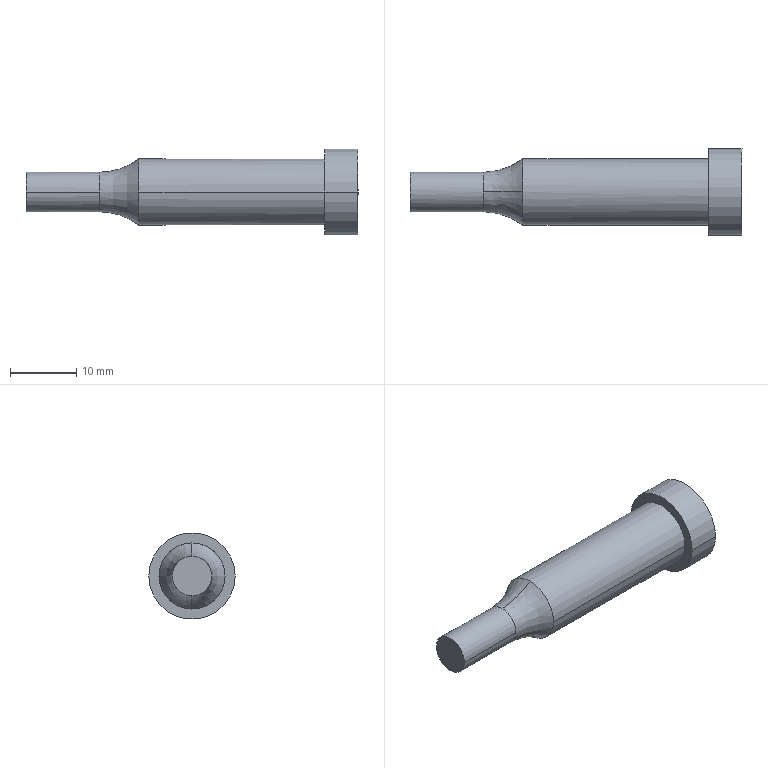Part | STEP file | CHAY 6X10X50.dwg | 1 solid | 11 faces | box 50 x 13 x 13 mm | volume 3399 mm3 | cylinder 6 | plane 3 | spline 2 | commonest cylinder face diameters 5.95 x2 9.95 x2 13 x2
STEP:
#1=CARTESIAN_POINT('',(0.,0.,0.));
#2=DIRECTION('',(0.,0.,1.));
#3=DIRECTION('',(1.,0.,0.));
#4=AXIS2_PLACEMENT_3D('',#1,#2,#3);
#5=CARTESIAN_POINT('',(-39.,2.975,0.));
#6=VERTEX_POINT('',#5);
#7=CARTESIAN_POINT('',(-39.,0.,-2.975));
#8=VERTEX_POINT('',#7);
#9=CARTESIAN_POINT('',(-39.,0.,0.));
#10=DIRECTION('',(-1.,0.,0.));
#11=DIRECTION('',(0.,0.,-1.));
#12=AXIS2_PLACEMENT_3D('',#9,#10,#11);
#13=CIRCLE('',#12,2.975);
#14=CARTESIAN_POINT('',(-39.,0.,-2.975));
#15=CARTESIAN_POINT('',(-39.,5.95,-2.975));
#16=CARTESIAN_POINT('',(-39.,5.95,2.975));
#17=CARTESIAN_POINT('',(-39.,0.,2.975));
#18=CARTESIAN_POINT('',(-36.817,0.,-2.975));
#19=CARTESIAN_POINT('',(-36.817,5.95,-2.975));
#20=CARTESIAN_POINT('',(-36.817,5.95,2.975));
#21=CARTESIAN_POINT('',(-36.817,0.,2.975));
#22=CARTESIAN_POINT('',(-34.746,0.,-3.665));
#23=CARTESIAN_POINT('',(-34.746,7.331,-3.665));
#24=CARTESIAN_POINT('',(-34.746,7.331,3.665));
#25=CARTESIAN_POINT('',(-34.746,0.,3.665));
#26=CARTESIAN_POINT('',(-33.,0.,-4.975));
#27=CARTESIAN_POINT('',(-33.,9.95,-4.975));
#28=CARTESIAN_POINT('',(-33.,9.95,4.975));
#29=CARTESIAN_POINT('',(-33.,0.,4.975));
#30=(BOUNDED_SURFACE()B_SPLINE_SURFACE(3,3,((#14,#15,#16,#17),(#18,#19,#20,#21),(#22,#23,#24,#25),(#26,#27,#28,#29)),.UNSPECIFIED.,.F.,.F.,.F.)B_SPLINE_SURFACE_WITH_KNOTS((4,4),(4,4),(0.,1.),(0.,1.),.PIECEWISE_BEZIER_KNOTS.)GEOMETRIC_REPRESENTATION_ITEM()RATIONAL_B_SPLINE_SURFACE(((1.,0.3333,0.3333,1.),(0.9658,0.3219,0.3219,0.9658),(0.9658,0.3219,0.3219,0.9658),(1.,0.3333,0.3333,1.)))REPRESENTATION_ITEM('')SURFACE());
#31=CARTESIAN_POINT('',(0.,0.5));
#32=CARTESIAN_POINT('',(0.,0.494));
#33=CARTESIAN_POINT('',(0.,0.4822));
#34=CARTESIAN_POINT('',(0.,0.4643));
#35=CARTESIAN_POINT('',(0.,0.4463));
#36=CARTESIAN_POINT('',(0.,0.4281));
#37=CARTESIAN_POINT('',(0.,0.4098));
#38=CARTESIAN_POINT('',(0.,0.3913));
#39=CARTESIAN_POINT('',(0.,0.3724));
#40=CARTESIAN_POINT('',(0.,0.3533));
#41=CARTESIAN_POINT('',(0.,0.3337));
#42=CARTESIAN_POINT('',(0.,0.3136));
#43=CARTESIAN_POINT('',(0.,0.293));
#44=CARTESIAN_POINT('',(0.,0.2718));
#45=CARTESIAN_POINT('',(0.,0.2499));
#46=CARTESIAN_POINT('',(0.,0.2271));
#47=CARTESIAN_POINT('',(0.,0.2035));
#48=CARTESIAN_POINT('',(0.,0.1789));
#49=CARTESIAN_POINT('',(0.,0.1531));
#50=CARTESIAN_POINT('',(0.,0.126));
#51=CARTESIAN_POINT('',(0.,0.09736));
#52=CARTESIAN_POINT('',(0.,0.06707));
#53=CARTESIAN_POINT('',(0.,0.03485));
#54=CARTESIAN_POINT('',(0.,0.0119));
#55=CARTESIAN_POINT('',(0.,0.));
#56=B_SPLINE_CURVE_WITH_KNOTS('',3,(#31,#32,#33,#34,#35,#36,#37,#38,#39,#40,#41,#42,#43,#44,#45,#46,#47,#48,#49,#50,#51,#52,#53,#54,#55),.UNSPECIFIED.,.F.,.F.,(4,1,1,1,1,1,1,1,1,1,1,1,1,1,1,1,1,1,1,1,1,1,4),(4.712,4.784,4.855,4.927,4.998,5.069,5.141,5.212,5.284,5.355,5.426,5.498,5.569,5.641,5.712,5.783,5.855,5.926,5.998,6.069,6.14,6.212,6.283),.QUASI_UNIFORM_KNOTS.);
#57=(GEOMETRIC_REPRESENTATION_CONTEXT(2)PARAMETRIC_REPRESENTATION_CONTEXT()REPRESENTATION_CONTEXT('',''));
#58=DEFINITIONAL_REPRESENTATION('',(#56),#57);
#59=PCURVE('',#30,#58);
#60=CARTESIAN_POINT('',(-44.5,0.,0.));
#61=DIRECTION('',(1.,0.,0.));
#62=DIRECTION('',(0.,1.,0.));
#63=AXIS2_PLACEMENT_3D('',#60,#61,#62);
#64=CYLINDRICAL_SURFACE('',#63,2.975);
#65=CARTESIAN_POINT('',(10.996,5.5));
#66=DIRECTION('',(-1.,0.));
#67=VECTOR('',#66,1.);
#68=LINE('',#65,#67);
#69=(GEOMETRIC_REPRESENTATION_CONTEXT(2)PARAMETRIC_REPRESENTATION_CONTEXT()REPRESENTATION_CONTEXT('',''));
#70=DEFINITIONAL_REPRESENTATION('',(#68),#69);
#71=PCURVE('',#64,#70);
#72=SURFACE_CURVE('',#13,(#59,#71),.PCURVE_S1.);
#73=EDGE_CURVE('',#6,#8,#72,.T.);
#74=ORIENTED_EDGE('',*,*,#73,.T.);
#75=CARTESIAN_POINT('',(-33.,0.,-4.975));
#76=VERTEX_POINT('',#75);
#77=CARTESIAN_POINT('',(-39.,0.,-12.975));
#78=DIRECTION('',(0.,1.,0.));
#79=DIRECTION('',(0.,0.,-1.));
#80=AXIS2_PLACEMENT_3D('',#77,#78,#79);
#81=CIRCLE('',#80,10.);
#82=CARTESIAN_POINT('',(0.,0.));
#83=CARTESIAN_POINT('',(0.01542,0.));
#84=CARTESIAN_POINT('',(0.04618,0.));
#85=CARTESIAN_POINT('',(0.09212,0.));
#86=CARTESIAN_POINT('',(0.1379,0.));
#87=CARTESIAN_POINT('',(0.1835,0.));
#88=CARTESIAN_POINT('',(0.229,0.));
#89=CARTESIAN_POINT('',(0.2743,0.));
#90=CARTESIAN_POINT('',(0.3196,0.));
#91=CARTESIAN_POINT('',(0.3647,0.));
#92=CARTESIAN_POINT('',(0.4099,0.));
#93=CARTESIAN_POINT('',(0.4549,0.));
#94=CARTESIAN_POINT('',(0.5,0.));
#95=CARTESIAN_POINT('',(0.5451,0.));
#96=CARTESIAN_POINT('',(0.5901,0.));
#97=CARTESIAN_POINT('',(0.6353,0.));
#98=CARTESIAN_POINT('',(0.6804,0.));
#99=CARTESIAN_POINT('',(0.7257,0.));
#100=CARTESIAN_POINT('',(0.771,0.));
#101=CARTESIAN_POINT('',(0.8165,0.));
#102=CARTESIAN_POINT('',(0.8621,0.));
#103=CARTESIAN_POINT('',(0.9079,0.));
#104=CARTESIAN_POINT('',(0.9538,0.));
#105=CARTESIAN_POINT('',(0.9846,0.));
#106=CARTESIAN_POINT('',(1.,0.));
#107=B_SPLINE_CURVE_WITH_KNOTS('',3,(#82,#83,#84,#85,#86,#87,#88,#89,#90,#91,#92,#93,#94,#95,#96,#97,#98,#99,#100,#101,#102,#103,#104,#105,#106),.UNSPECIFIED.,.F.,.F.,(4,1,1,1,1,1,1,1,1,1,1,1,1,1,1,1,1,1,1,1,1,1,4),(3.142,3.171,3.2,3.229,3.259,3.288,3.317,3.346,3.376,3.405,3.434,3.463,3.493,3.522,3.551,3.58,3.61,3.639,3.668,3.697,3.727,3.756,3.785),.QUASI_UNIFORM_KNOTS.);
#108=(GEOMETRIC_REPRESENTATION_CONTEXT(2)PARAMETRIC_REPRESENTATION_CONTEXT()REPRESENTATION_CONTEXT('',''));
#109=DEFINITIONAL_REPRESENTATION('',(#107),#108);
#110=PCURVE('',#30,#109);
#111=CARTESIAN_POINT('',(-39.,0.,2.975));
#112=CARTESIAN_POINT('',(-39.,-5.95,2.975));
#113=CARTESIAN_POINT('',(-39.,-5.95,-2.975));
#114=CARTESIAN_POINT('',(-39.,0.,-2.975));
#115=CARTESIAN_POINT('',(-36.817,0.,2.975));
#116=CARTESIAN_POINT('',(-36.817,-5.95,2.975));
#117=CARTESIAN_POINT('',(-36.817,-5.95,-2.975));
#118=CARTESIAN_POINT('',(-36.817,0.,-2.975));
#119=CARTESIAN_POINT('',(-34.746,0.,3.665));
#120=CARTESIAN_POINT('',(-34.746,-7.331,3.665));
#121=CARTESIAN_POINT('',(-34.746,-7.331,-3.665));
#122=CARTESIAN_POINT('',(-34.746,0.,-3.665));
#123=CARTESIAN_POINT('',(-33.,0.,4.975));
#124=CARTESIAN_POINT('',(-33.,-9.95,4.975));
#125=CARTESIAN_POINT('',(-33.,-9.95,-4.975));
#126=CARTESIAN_POINT('',(-33.,0.,-4.975));
#127=(BOUNDED_SURFACE()B_SPLINE_SURFACE(3,3,((#111,#112,#113,#114),(#115,#116,#117,#118),(#119,#120,#121,#122),(#123,#124,#125,#126)),.UNSPECIFIED.,.F.,.F.,.F.)B_SPLINE_SURFACE_WITH_KNOTS((4,4),(4,4),(0.,1.),(0.,1.),.PIECEWISE_BEZIER_KNOTS.)GEOMETRIC_REPRESENTATION_ITEM()RATIONAL_B_SPLINE_SURFACE(((1.,0.3333,0.3333,1.),(0.9658,0.3219,0.3219,0.9658),(0.9658,0.3219,0.3219,0.9658),(1.,0.3333,0.3333,1.)))REPRESENTATION_ITEM('')SURFACE());
#128=CARTESIAN_POINT('',(0.,1.));
#129=CARTESIAN_POINT('',(0.01542,1.));
#130=CARTESIAN_POINT('',(0.04618,1.));
#131=CARTESIAN_POINT('',(0.09212,1.));
#132=CARTESIAN_POINT('',(0.1379,1.));
#133=CARTESIAN_POINT('',(0.1835,1.));
#134=CARTESIAN_POINT('',(0.229,1.));
#135=CARTESIAN_POINT('',(0.2743,1.));
#136=CARTESIAN_POINT('',(0.3196,1.));
#137=CARTESIAN_POINT('',(0.3647,1.));
#138=CARTESIAN_POINT('',(0.4099,1.));
#139=CARTESIAN_POINT('',(0.4549,1.));
#140=CARTESIAN_POINT('',(0.5,1.));
#141=CARTESIAN_POINT('',(0.5451,1.));
#142=CARTESIAN_POINT('',(0.5901,1.));
#143=CARTESIAN_POINT('',(0.6353,1.));
#144=CARTESIAN_POINT('',(0.6804,1.));
#145=CARTESIAN_POINT('',(0.7257,1.));
#146=CARTESIAN_POINT('',(0.771,1.));
#147=CARTESIAN_POINT('',(0.8165,1.));
#148=CARTESIAN_POINT('',(0.8621,1.));
#149=CARTESIAN_POINT('',(0.9079,1.));
#150=CARTESIAN_POINT('',(0.9538,1.));
#151=CARTESIAN_POINT('',(0.9846,1.));
#152=CARTESIAN_POINT('',(1.,1.));
#153=B_SPLINE_CURVE_WITH_KNOTS('',3,(#128,#129,#130,#131,#132,#133,#134,#135,#136,#137,#138,#139,#140,#141,#142,#143,#144,#145,#146,#147,#148,#149,#150,#151,#152),.UNSPECIFIED.,.F.,.F.,(4,1,1,1,1,1,1,1,1,1,1,1,1,1,1,1,1,1,1,1,1,1,4),(3.142,3.171,3.2,3.229,3.259,3.288,3.317,3.346,3.376,3.405,3.434,3.463,3.493,3.522,3.551,3.58,3.61,3.639,3.668,3.697,3.727,3.756,3.785),.QUASI_UNIFORM_KNOTS.);
#154=(GEOMETRIC_REPRESENTATION_CONTEXT(2)PARAMETRIC_REPRESENTATION_CONTEXT()REPRESENTATION_CONTEXT('',''));
#155=DEFINITIONAL_REPRESENTATION('',(#153),#154);
#156=PCURVE('',#127,#155);
#157=SURFACE_CURVE('',#81,(#110,#156),.PCURVE_S1.);
#158=EDGE_CURVE('',#8,#76,#157,.T.);
#159=ORIENTED_EDGE('',*,*,#158,.T.);
#160=CARTESIAN_POINT('',(-33.,4.975,0.));
#161=VERTEX_POINT('',#160);
#162=CARTESIAN_POINT('',(-33.,0.,0.));
#163=DIRECTION('',(1.,0.,0.));
#164=DIRECTION('',(0.,1.,0.));
#165=AXIS2_PLACEMENT_3D('',#162,#163,#164);
#166=CIRCLE('',#165,4.975);
#167=CARTESIAN_POINT('',(1.,0.));
#168=CARTESIAN_POINT('',(1.,0.0119));
#169=CARTESIAN_POINT('',(1.,0.03485));
#170=CARTESIAN_POINT('',(1.,0.06707));
#171=CARTESIAN_POINT('',(1.,0.09736));
#172=CARTESIAN_POINT('',(1.,0.126));
#173=CARTESIAN_POINT('',(1.,0.1531));
#174=CARTESIAN_POINT('',(1.,0.1789));
#175=CARTESIAN_POINT('',(1.,0.2035));
#176=CARTESIAN_POINT('',(1.,0.2271));
#177=CARTESIAN_POINT('',(1.,0.2499));
#178=CARTESIAN_POINT('',(1.,0.2718));
#179=CARTESIAN_POINT('',(1.,0.293));
#180=CARTESIAN_POINT('',(1.,0.3136));
#181=CARTESIAN_POINT('',(1.,0.3337));
#182=CARTESIAN_POINT('',(1.,0.3533));
#183=CARTESIAN_POINT('',(1.,0.3724));
#184=CARTESIAN_POINT('',(1.,0.3913));
#185=CARTESIAN_POINT('',(1.,0.4098));
#186=CARTESIAN_POINT('',(1.,0.4281));
#187=CARTESIAN_POINT('',(1.,0.4463));
#188=CARTESIAN_POINT('',(1.,0.4643));
#189=CARTESIAN_POINT('',(1.,0.4822));
#190=CARTESIAN_POINT('',(1.,0.494));
#191=CARTESIAN_POINT('',(1.,0.5));
#192=B_SPLINE_CURVE_WITH_KNOTS('',3,(#167,#168,#169,#170,#171,#172,#173,#174,#175,#176,#177,#178,#179,#180,#181,#182,#183,#184,#185,#186,#187,#188,#189,#190,#191),.UNSPECIFIED.,.F.,.F.,(4,1,1,1,1,1,1,1,1,1,1,1,1,1,1,1,1,1,1,1,1,1,4),(4.712,4.784,4.855,4.927,4.998,5.069,5.141,5.212,5.284,5.355,5.426,5.498,5.569,5.641,5.712,5.783,5.855,5.926,5.998,6.069,6.14,6.212,6.283),.QUASI_UNIFORM_KNOTS.);
#193=(GEOMETRIC_REPRESENTATION_CONTEXT(2)PARAMETRIC_REPRESENTATION_CONTEXT()REPRESENTATION_CONTEXT('',''));
#194=DEFINITIONAL_REPRESENTATION('',(#192),#193);
#195=PCURVE('',#30,#194);
#196=CARTESIAN_POINT('',(-19.,0.,0.));
#197=DIRECTION('',(1.,0.,0.));
#198=DIRECTION('',(0.,1.,0.));
#199=AXIS2_PLACEMENT_3D('',#196,#197,#198);
#200=CYLINDRICAL_SURFACE('',#199,4.975);
#201=CARTESIAN_POINT('',(0.,-14.));
#202=DIRECTION('',(1.,0.));
#203=VECTOR('',#202,1.);
#204=LINE('',#201,#203);
#205=(GEOMETRIC_REPRESENTATION_CONTEXT(2)PARAMETRIC_REPRESENTATION_CONTEXT()REPRESENTATION_CONTEXT('',''));
#206=DEFINITIONAL_REPRESENTATION('',(#204),#205);
#207=PCURVE('',#200,#206);
#208=SURFACE_CURVE('',#166,(#195,#207),.PCURVE_S1.);
#209=EDGE_CURVE('',#76,#161,#208,.T.);
#210=ORIENTED_EDGE('',*,*,#209,.T.);
#211=CARTESIAN_POINT('',(-33.,0.,4.975));
#212=VERTEX_POINT('',#211);
#213=CARTESIAN_POINT('',(-33.,0.,0.));
#214=DIRECTION('',(1.,0.,0.));
#215=DIRECTION('',(0.,1.,0.));
#216=AXIS2_PLACEMENT_3D('',#213,#214,#215);
#217=CIRCLE('',#216,4.975);
#218=CARTESIAN_POINT('',(1.,0.5));
#219=CARTESIAN_POINT('',(1.,0.506));
#220=CARTESIAN_POINT('',(1.,0.5178));
#221=CARTESIAN_POINT('',(1.,0.5357));
#222=CARTESIAN_POINT('',(1.,0.5537));
#223=CARTESIAN_POINT('',(1.,0.5719));
#224=CARTESIAN_POINT('',(1.,0.5902));
#225=CARTESIAN_POINT('',(1.,0.6087));
#226=CARTESIAN_POINT('',(1.,0.6276));
#227=CARTESIAN_POINT('',(1.,0.6467));
#228=CARTESIAN_POINT('',(1.,0.6663));
#229=CARTESIAN_POINT('',(1.,0.6864));
#230=CARTESIAN_POINT('',(1.,0.707));
#231=CARTESIAN_POINT('',(1.,0.7282));
#232=CARTESIAN_POINT('',(1.,0.7501));
#233=CARTESIAN_POINT('',(1.,0.7729));
#234=CARTESIAN_POINT('',(1.,0.7965));
#235=CARTESIAN_POINT('',(1.,0.8211));
#236=CARTESIAN_POINT('',(1.,0.8469));
#237=CARTESIAN_POINT('',(1.,0.874));
#238=CARTESIAN_POINT('',(1.,0.9026));
#239=CARTESIAN_POINT('',(1.,0.9329));
#240=CARTESIAN_POINT('',(1.,0.9651));
#241=CARTESIAN_POINT('',(1.,0.9881));
#242=CARTESIAN_POINT('',(1.,1.));
#243=B_SPLINE_CURVE_WITH_KNOTS('',3,(#218,#219,#220,#221,#222,#223,#224,#225,#226,#227,#228,#229,#230,#231,#232,#233,#234,#235,#236,#237,#238,#239,#240,#241,#242),.UNSPECIFIED.,.F.,.F.,(4,1,1,1,1,1,1,1,1,1,1,1,1,1,1,1,1,1,1,1,1,1,4),(0.,0.0714,0.1428,0.2142,0.2856,0.357,0.4284,0.4998,0.5712,0.6426,0.714,0.7854,0.8568,0.9282,0.9996,1.071,1.142,1.214,1.285,1.357,1.428,1.499,1.571),.QUASI_UNIFORM_KNOTS.);
#244=(GEOMETRIC_REPRESENTATION_CONTEXT(2)PARAMETRIC_REPRESENTATION_CONTEXT()REPRESENTATION_CONTEXT('',''));
#245=DEFINITIONAL_REPRESENTATION('',(#243),#244);
#246=PCURVE('',#30,#245);
#247=CARTESIAN_POINT('',(-19.,0.,0.));
#248=DIRECTION('',(1.,0.,0.));
#249=DIRECTION('',(0.,1.,0.));
#250=AXIS2_PLACEMENT_3D('',#247,#248,#249);
#251=CYLINDRICAL_SURFACE('',#250,4.975);
#252=CARTESIAN_POINT('',(0.,-14.));
#253=DIRECTION('',(1.,0.));
#254=VECTOR('',#253,1.);
#255=LINE('',#252,#254);
#256=(GEOMETRIC_REPRESENTATION_CONTEXT(2)PARAMETRIC_REPRESENTATION_CONTEXT()REPRESENTATION_CONTEXT('',''));
#257=DEFINITIONAL_REPRESENTATION('',(#255),#256);
#258=PCURVE('',#251,#257);
#259=SURFACE_CURVE('',#217,(#246,#258),.PCURVE_S1.);
#260=EDGE_CURVE('',#161,#212,#259,.T.);
#261=ORIENTED_EDGE('',*,*,#260,.T.);
#262=CARTESIAN_POINT('',(-39.,0.,2.975));
#263=VERTEX_POINT('',#262);
#264=CARTESIAN_POINT('',(-39.,0.,12.975));
#265=DIRECTION('',(0.,-1.,0.));
#266=DIRECTION('',(0.,0.,1.));
#267=AXIS2_PLACEMENT_3D('',#264,#265,#266);
#268=CIRCLE('',#267,10.);
#269=CARTESIAN_POINT('',(0.,1.));
#270=CARTESIAN_POINT('',(0.01542,1.));
#271=CARTESIAN_POINT('',(0.04618,1.));
#272=CARTESIAN_POINT('',(0.09212,1.));
#273=CARTESIAN_POINT('',(0.1379,1.));
#274=CARTESIAN_POINT('',(0.1835,1.));
#275=CARTESIAN_POINT('',(0.229,1.));
#276=CARTESIAN_POINT('',(0.2743,1.));
#277=CARTESIAN_POINT('',(0.3196,1.));
#278=CARTESIAN_POINT('',(0.3647,1.));
#279=CARTESIAN_POINT('',(0.4099,1.));
#280=CARTESIAN_POINT('',(0.4549,1.));
#281=CARTESIAN_POINT('',(0.5,1.));
#282=CARTESIAN_POINT('',(0.5451,1.));
#283=CARTESIAN_POINT('',(0.5901,1.));
#284=CARTESIAN_POINT('',(0.6353,1.));
#285=CARTESIAN_POINT('',(0.6804,1.));
#286=CARTESIAN_POINT('',(0.7257,1.));
#287=CARTESIAN_POINT('',(0.771,1.));
#288=CARTESIAN_POINT('',(0.8165,1.));
#289=CARTESIAN_POINT('',(0.8621,1.));
#290=CARTESIAN_POINT('',(0.9079,1.));
#291=CARTESIAN_POINT('',(0.9538,1.));
#292=CARTESIAN_POINT('',(0.9846,1.));
#293=CARTESIAN_POINT('',(1.,1.));
#294=B_SPLINE_CURVE_WITH_KNOTS('',3,(#269,#270,#271,#272,#273,#274,#275,#276,#277,#278,#279,#280,#281,#282,#283,#284,#285,#286,#287,#288,#289,#290,#291,#292,#293),.UNSPECIFIED.,.F.,.F.,(4,1,1,1,1,1,1,1,1,1,1,1,1,1,1,1,1,1,1,1,1,1,4),(3.142,3.171,3.2,3.229,3.259,3.288,3.317,3.346,3.376,3.405,3.434,3.463,3.493,3.522,3.551,3.58,3.61,3.639,3.668,3.697,3.727,3.756,3.785),.QUASI_UNIFORM_KNOTS.);
#295=(GEOMETRIC_REPRESENTATION_CONTEXT(2)PARAMETRIC_REPRESENTATION_CONTEXT()REPRESENTATION_CONTEXT('',''));
#296=DEFINITIONAL_REPRESENTATION('',(#294),#295);
#297=PCURVE('',#30,#296);
#298=CARTESIAN_POINT('',(0.,0.));
#299=CARTESIAN_POINT('',(0.01542,0.));
#300=CARTESIAN_POINT('',(0.04618,0.));
#301=CARTESIAN_POINT('',(0.09212,0.));
#302=CARTESIAN_POINT('',(0.1379,0.));
#303=CARTESIAN_POINT('',(0.1835,0.));
#304=CARTESIAN_POINT('',(0.229,0.));
#305=CARTESIAN_POINT('',(0.2743,0.));
#306=CARTESIAN_POINT('',(0.3196,0.));
#307=CARTESIAN_POINT('',(0.3647,0.));
#308=CARTESIAN_POINT('',(0.4099,0.));
#309=CARTESIAN_POINT('',(0.4549,0.));
#310=CARTESIAN_POINT('',(0.5,0.));
#311=CARTESIAN_POINT('',(0.5451,0.));
#312=CARTESIAN_POINT('',(0.5901,0.));
#313=CARTESIAN_POINT('',(0.6353,0.));
#314=CARTESIAN_POINT('',(0.6804,0.));
#315=CARTESIAN_POINT('',(0.7257,0.));
#316=CARTESIAN_POINT('',(0.771,0.));
#317=CARTESIAN_POINT('',(0.8165,0.));
#318=CARTESIAN_POINT('',(0.8621,0.));
#319=CARTESIAN_POINT('',(0.9079,0.));
#320=CARTESIAN_POINT('',(0.9538,0.));
#321=CARTESIAN_POINT('',(0.9846,0.));
#322=CARTESIAN_POINT('',(1.,0.));
#323=B_SPLINE_CURVE_WITH_KNOTS('',3,(#298,#299,#300,#301,#302,#303,#304,#305,#306,#307,#308,#309,#310,#311,#312,#313,#314,#315,#316,#317,#318,#319,#320,#321,#322),.UNSPECIFIED.,.F.,.F.,(4,1,1,1,1,1,1,1,1,1,1,1,1,1,1,1,1,1,1,1,1,1,4),(3.142,3.171,3.2,3.229,3.259,3.288,3.317,3.346,3.376,3.405,3.434,3.463,3.493,3.522,3.551,3.58,3.61,3.639,3.668,3.697,3.727,3.756,3.785),.QUASI_UNIFORM_KNOTS.);
#324=(GEOMETRIC_REPRESENTATION_CONTEXT(2)PARAMETRIC_REPRESENTATION_CONTEXT()REPRESENTATION_CONTEXT('',''));
#325=DEFINITIONAL_REPRESENTATION('',(#323),#324);
#326=PCURVE('',#127,#325);
#327=SURFACE_CURVE('',#268,(#297,#326),.PCURVE_S1.);
#328=EDGE_CURVE('',#263,#212,#327,.T.);
#329=ORIENTED_EDGE('',*,*,#328,.F.);
#330=CARTESIAN_POINT('',(-39.,0.,0.));
#331=DIRECTION('',(-1.,0.,0.));
#332=DIRECTION('',(0.,0.,-1.));
#333=AXIS2_PLACEMENT_3D('',#330,#331,#332);
#334=CIRCLE('',#333,2.975);
#335=CARTESIAN_POINT('',(0.,1.));
#336=CARTESIAN_POINT('',(0.,0.9881));
#337=CARTESIAN_POINT('',(0.,0.9651));
#338=CARTESIAN_POINT('',(0.,0.9329));
#339=CARTESIAN_POINT('',(0.,0.9026));
#340=CARTESIAN_POINT('',(0.,0.874));
#341=CARTESIAN_POINT('',(0.,0.8469));
#342=CARTESIAN_POINT('',(0.,0.8211));
#343=CARTESIAN_POINT('',(0.,0.7965));
#344=CARTESIAN_POINT('',(0.,0.7729));
#345=CARTESIAN_POINT('',(0.,0.7501));
#346=CARTESIAN_POINT('',(0.,0.7282));
#347=CARTESIAN_POINT('',(0.,0.707));
#348=CARTESIAN_POINT('',(0.,0.6864));
#349=CARTESIAN_POINT('',(0.,0.6663));
#350=CARTESIAN_POINT('',(0.,0.6467));
#351=CARTESIAN_POINT('',(0.,0.6276));
#352=CARTESIAN_POINT('',(0.,0.6087));
#353=CARTESIAN_POINT('',(0.,0.5902));
#354=CARTESIAN_POINT('',(0.,0.5719));
#355=CARTESIAN_POINT('',(0.,0.5537));
#356=CARTESIAN_POINT('',(0.,0.5357));
#357=CARTESIAN_POINT('',(0.,0.5178));
#358=CARTESIAN_POINT('',(0.,0.506));
#359=CARTESIAN_POINT('',(0.,0.5));
#360=B_SPLINE_CURVE_WITH_KNOTS('',3,(#335,#336,#337,#338,#339,#340,#341,#342,#343,#344,#345,#346,#347,#348,#349,#350,#351,#352,#353,#354,#355,#356,#357,#358,#359),.UNSPECIFIED.,.F.,.F.,(4,1,1,1,1,1,1,1,1,1,1,1,1,1,1,1,1,1,1,1,1,1,4),(3.142,3.213,3.284,3.356,3.427,3.499,3.57,3.641,3.713,3.784,3.856,3.927,3.998,4.07,4.141,4.213,4.284,4.355,4.427,4.498,4.57,4.641,4.712),.QUASI_UNIFORM_KNOTS.);
#361=(GEOMETRIC_REPRESENTATION_CONTEXT(2)PARAMETRIC_REPRESENTATION_CONTEXT()REPRESENTATION_CONTEXT('',''));
#362=DEFINITIONAL_REPRESENTATION('',(#360),#361);
#363=PCURVE('',#30,#362);
#364=CARTESIAN_POINT('',(-44.5,0.,0.));
#365=DIRECTION('',(1.,0.,0.));
#366=DIRECTION('',(0.,1.,0.));
#367=AXIS2_PLACEMENT_3D('',#364,#365,#366);
#368=CYLINDRICAL_SURFACE('',#367,2.975);
#369=CARTESIAN_POINT('',(4.712,5.5));
#370=DIRECTION('',(-1.,0.));
#371=VECTOR('',#370,1.);
#372=LINE('',#369,#371);
#373=(GEOMETRIC_REPRESENTATION_CONTEXT(2)PARAMETRIC_REPRESENTATION_CONTEXT()REPRESENTATION_CONTEXT('',''));
#374=DEFINITIONAL_REPRESENTATION('',(#372),#373);
#375=PCURVE('',#368,#374);
#376=SURFACE_CURVE('',#334,(#363,#375),.PCURVE_S1.);
#377=EDGE_CURVE('',#263,#6,#376,.T.);
#378=ORIENTED_EDGE('',*,*,#377,.T.);
#379=EDGE_LOOP('',(#74,#159,#210,#261,#329,#378));
#380=FACE_BOUND('',#379,.F.);
#381=ADVANCED_FACE('',(#380),#30,.F.);
#382=ORIENTED_EDGE('',*,*,#260,.T.);
#383=CARTESIAN_POINT('',(-33.,-4.975,0.));
#384=VERTEX_POINT('',#383);
#385=CARTESIAN_POINT('',(-33.,0.,0.));
#386=DIRECTION('',(1.,0.,0.));
#387=DIRECTION('',(0.,1.,0.));
#388=AXIS2_PLACEMENT_3D('',#385,#386,#387);
#389=CIRCLE('',#388,4.975);
#390=CARTESIAN_POINT('',(0.,-14.));
#391=DIRECTION('',(1.,0.));
#392=VECTOR('',#391,1.);
#393=LINE('',#390,#392);
#394=(GEOMETRIC_REPRESENTATION_CONTEXT(2)PARAMETRIC_REPRESENTATION_CONTEXT()REPRESENTATION_CONTEXT('',''));
#395=DEFINITIONAL_REPRESENTATION('',(#393),#394);
#396=PCURVE('',#251,#395);
#397=CARTESIAN_POINT('',(1.,0.));
#398=CARTESIAN_POINT('',(1.,0.0119));
#399=CARTESIAN_POINT('',(1.,0.03485));
#400=CARTESIAN_POINT('',(1.,0.06707));
#401=CARTESIAN_POINT('',(1.,0.09736));
#402=CARTESIAN_POINT('',(1.,0.126));
#403=CARTESIAN_POINT('',(1.,0.1531));
#404=CARTESIAN_POINT('',(1.,0.1789));
#405=CARTESIAN_POINT('',(1.,0.2035));
#406=CARTESIAN_POINT('',(1.,0.2271));
#407=CARTESIAN_POINT('',(1.,0.2499));
#408=CARTESIAN_POINT('',(1.,0.2718));
#409=CARTESIAN_POINT('',(1.,0.293));
#410=CARTESIAN_POINT('',(1.,0.3136));
#411=CARTESIAN_POINT('',(1.,0.3337));
#412=CARTESIAN_POINT('',(1.,0.3533));
#413=CARTESIAN_POINT('',(1.,0.3724));
#414=CARTESIAN_POINT('',(1.,0.3913));
#415=CARTESIAN_POINT('',(1.,0.4098));
#416=CARTESIAN_POINT('',(1.,0.4281));
#417=CARTESIAN_POINT('',(1.,0.4463));
#418=CARTESIAN_POINT('',(1.,0.4643));
#419=CARTESIAN_POINT('',(1.,0.4822));
#420=CARTESIAN_POINT('',(1.,0.494));
#421=CARTESIAN_POINT('',(1.,0.5));
#422=B_SPLINE_CURVE_WITH_KNOTS('',3,(#397,#398,#399,#400,#401,#402,#403,#404,#405,#406,#407,#408,#409,#410,#411,#412,#413,#414,#415,#416,#417,#418,#419,#420,#421),.UNSPECIFIED.,.F.,.F.,(4,1,1,1,1,1,1,1,1,1,1,1,1,1,1,1,1,1,1,1,1,1,4),(1.571,1.642,1.714,1.785,1.856,1.928,1.999,2.071,2.142,2.213,2.285,2.356,2.428,2.499,2.57,2.642,2.713,2.785,2.856,2.927,2.999,3.07,3.142),.QUASI_UNIFORM_KNOTS.);
#423=(GEOMETRIC_REPRESENTATION_CONTEXT(2)PARAMETRIC_REPRESENTATION_CONTEXT()REPRESENTATION_CONTEXT('',''));
#424=DEFINITIONAL_REPRESENTATION('',(#422),#423);
#425=PCURVE('',#127,#424);
#426=SURFACE_CURVE('',#389,(#396,#425),.PCURVE_S1.);
#427=EDGE_CURVE('',#212,#384,#426,.T.);
#428=ORIENTED_EDGE('',*,*,#427,.T.);
#429=CARTESIAN_POINT('',(-5.,-4.975,0.));
#430=VERTEX_POINT('',#429);
#431=CARTESIAN_POINT('',(-19.,-4.975,0.));
#432=DIRECTION('',(1.,0.,0.));
#433=VECTOR('',#432,1.);
#434=LINE('',#431,#433);
#435=CARTESIAN_POINT('',(3.142,0.));
#436=DIRECTION('',(0.,1.));
#437=VECTOR('',#436,1.);
#438=LINE('',#435,#437);
#439=(GEOMETRIC_REPRESENTATION_CONTEXT(2)PARAMETRIC_REPRESENTATION_CONTEXT()REPRESENTATION_CONTEXT('',''));
#440=DEFINITIONAL_REPRESENTATION('',(#438),#439);
#441=PCURVE('',#251,#440);
#442=CARTESIAN_POINT('',(3.142,0.));
#443=DIRECTION('',(0.,1.));
#444=VECTOR('',#443,1.);
#445=LINE('',#442,#444);
#446=(GEOMETRIC_REPRESENTATION_CONTEXT(2)PARAMETRIC_REPRESENTATION_CONTEXT()REPRESENTATION_CONTEXT('',''));
#447=DEFINITIONAL_REPRESENTATION('',(#445),#446);
#448=PCURVE('',#200,#447);
#449=SURFACE_CURVE('',#434,(#441,#448),.PCURVE_S1.);
#450=EDGE_CURVE('',#384,#430,#449,.T.);
#451=ORIENTED_EDGE('',*,*,#450,.T.);
#452=CARTESIAN_POINT('',(-5.,4.975,0.));
#453=VERTEX_POINT('',#452);
#454=CARTESIAN_POINT('',(-5.,0.,0.));
#455=DIRECTION('',(-1.,0.,0.));
#456=DIRECTION('',(0.,1.,0.));
#457=AXIS2_PLACEMENT_3D('',#454,#455,#456);
#458=CIRCLE('',#457,4.975);
#459=CARTESIAN_POINT('',(6.283,14.));
#460=DIRECTION('',(-1.,0.));
#461=VECTOR('',#460,1.);
#462=LINE('',#459,#461);
#463=(GEOMETRIC_REPRESENTATION_CONTEXT(2)PARAMETRIC_REPRESENTATION_CONTEXT()REPRESENTATION_CONTEXT('',''));
#464=DEFINITIONAL_REPRESENTATION('',(#462),#463);
#465=PCURVE('',#251,#464);
#466=CARTESIAN_POINT('',(-5.,5.737,0.));
#467=DIRECTION('',(-1.,0.,0.));
#468=DIRECTION('',(0.,0.,1.));
#469=AXIS2_PLACEMENT_3D('',#466,#467,#468);
#470=PLANE('',#469);
#471=CARTESIAN_POINT('',(0.,-5.737));
#472=DIRECTION('',(0.,1.));
#473=AXIS2_PLACEMENT_2D('',#471,#472);
#474=CIRCLE('',#473,4.975);
#475=(GEOMETRIC_REPRESENTATION_CONTEXT(2)PARAMETRIC_REPRESENTATION_CONTEXT()REPRESENTATION_CONTEXT('',''));
#476=DEFINITIONAL_REPRESENTATION('',(#474),#475);
#477=PCURVE('',#470,#476);
#478=SURFACE_CURVE('',#458,(#465,#477),.PCURVE_S1.);
#479=EDGE_CURVE('',#430,#453,#478,.T.);
#480=ORIENTED_EDGE('',*,*,#479,.T.);
#481=CARTESIAN_POINT('',(-19.,4.975,0.));
#482=DIRECTION('',(1.,0.,0.));
#483=VECTOR('',#482,1.);
#484=LINE('',#481,#483);
#485=CARTESIAN_POINT('',(0.,0.));
#486=DIRECTION('',(0.,1.));
#487=VECTOR('',#486,1.);
#488=LINE('',#485,#487);
#489=(GEOMETRIC_REPRESENTATION_CONTEXT(2)PARAMETRIC_REPRESENTATION_CONTEXT()REPRESENTATION_CONTEXT('',''));
#490=DEFINITIONAL_REPRESENTATION('',(#488),#489);
#491=PCURVE('',#251,#490);
#492=CARTESIAN_POINT('',(6.283,0.));
#493=DIRECTION('',(0.,1.));
#494=VECTOR('',#493,1.);
#495=LINE('',#492,#494);
#496=(GEOMETRIC_REPRESENTATION_CONTEXT(2)PARAMETRIC_REPRESENTATION_CONTEXT()REPRESENTATION_CONTEXT('',''));
#497=DEFINITIONAL_REPRESENTATION('',(#495),#496);
#498=PCURVE('',#200,#497);
#499=SURFACE_CURVE('',#484,(#491,#498),.PCURVE_S1.);
#500=EDGE_CURVE('',#161,#453,#499,.T.);
#501=ORIENTED_EDGE('',*,*,#500,.F.);
#502=EDGE_LOOP('',(#382,#428,#451,#480,#501));
#503=FACE_BOUND('',#502,.T.);
#504=ADVANCED_FACE('',(#503),#251,.T.);
#505=CARTESIAN_POINT('',(-50.,2.975,0.));
#506=VERTEX_POINT('',#505);
#507=CARTESIAN_POINT('',(-50.,-2.975,0.));
#508=VERTEX_POINT('',#507);
#509=CARTESIAN_POINT('',(-50.,0.,0.));
#510=DIRECTION('',(1.,0.,0.));
#511=DIRECTION('',(0.,1.,0.));
#512=AXIS2_PLACEMENT_3D('',#509,#510,#511);
#513=CIRCLE('',#512,2.975);
#514=CARTESIAN_POINT('',(0.,-5.5));
#515=DIRECTION('',(1.,0.));
#516=VECTOR('',#515,1.);
#517=LINE('',#514,#516);
#518=(GEOMETRIC_REPRESENTATION_CONTEXT(2)PARAMETRIC_REPRESENTATION_CONTEXT()REPRESENTATION_CONTEXT('',''));
#519=DEFINITIONAL_REPRESENTATION('',(#517),#518);
#520=PCURVE('',#368,#519);
#521=CARTESIAN_POINT('',(-50.,1.487,0.));
#522=DIRECTION('',(-1.,0.,0.));
#523=DIRECTION('',(0.,0.,1.));
#524=AXIS2_PLACEMENT_3D('',#521,#522,#523);
#525=PLANE('',#524);
#526=CARTESIAN_POINT('',(0.,1.487));
#527=CARTESIAN_POINT('',(5.153,1.487));
#528=CARTESIAN_POINT('',(2.576,-2.975));
#529=CARTESIAN_POINT('',(0.,-7.437));
#530=CARTESIAN_POINT('',(-2.576,-2.975));
#531=CARTESIAN_POINT('',(-5.153,1.487));
#532=CARTESIAN_POINT('',(0.,1.487));
#533=(BOUNDED_CURVE()B_SPLINE_CURVE(2,(#526,#527,#528,#529,#530,#531,#532),.UNSPECIFIED.,.T.,.F.)B_SPLINE_CURVE_WITH_KNOTS((1,2,2,2,2,1),(-2.094,0.,2.094,4.189,6.283,8.378),.UNSPECIFIED.)CURVE()GEOMETRIC_REPRESENTATION_ITEM()RATIONAL_B_SPLINE_CURVE((1.,0.5,1.,0.5,1.,0.5,1.))REPRESENTATION_ITEM(''));
#534=(GEOMETRIC_REPRESENTATION_CONTEXT(2)PARAMETRIC_REPRESENTATION_CONTEXT()REPRESENTATION_CONTEXT('',''));
#535=DEFINITIONAL_REPRESENTATION('',(#533),#534);
#536=PCURVE('',#525,#535);
#537=SURFACE_CURVE('',#513,(#520,#536),.PCURVE_S1.);
#538=EDGE_CURVE('',#506,#508,#537,.T.);
#539=ORIENTED_EDGE('',*,*,#538,.T.);
#540=CARTESIAN_POINT('',(-39.,-2.975,0.));
#541=VERTEX_POINT('',#540);
#542=CARTESIAN_POINT('',(-44.5,-2.975,0.));
#543=DIRECTION('',(1.,0.,0.));
#544=VECTOR('',#543,1.);
#545=LINE('',#542,#544);
#546=CARTESIAN_POINT('',(3.142,0.));
#547=DIRECTION('',(0.,1.));
#548=VECTOR('',#547,1.);
#549=LINE('',#546,#548);
#550=(GEOMETRIC_REPRESENTATION_CONTEXT(2)PARAMETRIC_REPRESENTATION_CONTEXT()REPRESENTATION_CONTEXT('',''));
#551=DEFINITIONAL_REPRESENTATION('',(#549),#550);
#552=PCURVE('',#368,#551);
#553=CARTESIAN_POINT('',(3.142,0.));
#554=DIRECTION('',(0.,1.));
#555=VECTOR('',#554,1.);
#556=LINE('',#553,#555);
#557=(GEOMETRIC_REPRESENTATION_CONTEXT(2)PARAMETRIC_REPRESENTATION_CONTEXT()REPRESENTATION_CONTEXT('',''));
#558=DEFINITIONAL_REPRESENTATION('',(#556),#557);
#559=PCURVE('',#64,#558);
#560=SURFACE_CURVE('',#545,(#552,#559),.PCURVE_S1.);
#561=EDGE_CURVE('',#508,#541,#560,.T.);
#562=ORIENTED_EDGE('',*,*,#561,.T.);
#563=CARTESIAN_POINT('',(-39.,0.,0.));
#564=DIRECTION('',(-1.,0.,0.));
#565=DIRECTION('',(0.,0.,-1.));
#566=AXIS2_PLACEMENT_3D('',#563,#564,#565);
#567=CIRCLE('',#566,2.975);
#568=CARTESIAN_POINT('',(4.712,5.5));
#569=DIRECTION('',(-1.,0.));
#570=VECTOR('',#569,1.);
#571=LINE('',#568,#570);
#572=(GEOMETRIC_REPRESENTATION_CONTEXT(2)PARAMETRIC_REPRESENTATION_CONTEXT()REPRESENTATION_CONTEXT('',''));
#573=DEFINITIONAL_REPRESENTATION('',(#571),#572);
#574=PCURVE('',#368,#573);
#575=CARTESIAN_POINT('',(0.,0.5));
#576=CARTESIAN_POINT('',(0.,0.494));
#577=CARTESIAN_POINT('',(0.,0.4822));
#578=CARTESIAN_POINT('',(0.,0.4643));
#579=CARTESIAN_POINT('',(0.,0.4463));
#580=CARTESIAN_POINT('',(0.,0.4281));
#581=CARTESIAN_POINT('',(0.,0.4098));
#582=CARTESIAN_POINT('',(0.,0.3913));
#583=CARTESIAN_POINT('',(0.,0.3724));
#584=CARTESIAN_POINT('',(0.,0.3533));
#585=CARTESIAN_POINT('',(0.,0.3337));
#586=CARTESIAN_POINT('',(0.,0.3136));
#587=CARTESIAN_POINT('',(0.,0.293));
#588=CARTESIAN_POINT('',(0.,0.2718));
#589=CARTESIAN_POINT('',(0.,0.2499));
#590=CARTESIAN_POINT('',(0.,0.2271));
#591=CARTESIAN_POINT('',(0.,0.2035));
#592=CARTESIAN_POINT('',(0.,0.1789));
#593=CARTESIAN_POINT('',(0.,0.1531));
#594=CARTESIAN_POINT('',(0.,0.126));
#595=CARTESIAN_POINT('',(0.,0.09736));
#596=CARTESIAN_POINT('',(0.,0.06707));
#597=CARTESIAN_POINT('',(0.,0.03485));
#598=CARTESIAN_POINT('',(0.,0.0119));
#599=CARTESIAN_POINT('',(0.,0.));
#600=B_SPLINE_CURVE_WITH_KNOTS('',3,(#575,#576,#577,#578,#579,#580,#581,#582,#583,#584,#585,#586,#587,#588,#589,#590,#591,#592,#593,#594,#595,#596,#597,#598,#599),.UNSPECIFIED.,.F.,.F.,(4,1,1,1,1,1,1,1,1,1,1,1,1,1,1,1,1,1,1,1,1,1,4),(1.571,1.642,1.714,1.785,1.856,1.928,1.999,2.071,2.142,2.213,2.285,2.356,2.428,2.499,2.57,2.642,2.713,2.785,2.856,2.927,2.999,3.07,3.142),.QUASI_UNIFORM_KNOTS.);
#601=(GEOMETRIC_REPRESENTATION_CONTEXT(2)PARAMETRIC_REPRESENTATION_CONTEXT()REPRESENTATION_CONTEXT('',''));
#602=DEFINITIONAL_REPRESENTATION('',(#600),#601);
#603=PCURVE('',#127,#602);
#604=SURFACE_CURVE('',#567,(#574,#603),.PCURVE_S1.);
#605=EDGE_CURVE('',#541,#263,#604,.T.);
#606=ORIENTED_EDGE('',*,*,#605,.T.);
#607=ORIENTED_EDGE('',*,*,#377,.T.);
#608=CARTESIAN_POINT('',(-44.5,2.975,0.));
#609=DIRECTION('',(1.,0.,0.));
#610=VECTOR('',#609,1.);
#611=LINE('',#608,#610);
#612=CARTESIAN_POINT('',(0.,0.));
#613=DIRECTION('',(0.,1.));
#614=VECTOR('',#613,1.);
#615=LINE('',#612,#614);
#616=(GEOMETRIC_REPRESENTATION_CONTEXT(2)PARAMETRIC_REPRESENTATION_CONTEXT()REPRESENTATION_CONTEXT('',''));
#617=DEFINITIONAL_REPRESENTATION('',(#615),#616);
#618=PCURVE('',#368,#617);
#619=CARTESIAN_POINT('',(6.283,0.));
#620=DIRECTION('',(0.,1.));
#621=VECTOR('',#620,1.);
#622=LINE('',#619,#621);
#623=(GEOMETRIC_REPRESENTATION_CONTEXT(2)PARAMETRIC_REPRESENTATION_CONTEXT()REPRESENTATION_CONTEXT('',''));
#624=DEFINITIONAL_REPRESENTATION('',(#622),#623);
#625=PCURVE('',#64,#624);
#626=SURFACE_CURVE('',#611,(#618,#625),.PCURVE_S1.);
#627=EDGE_CURVE('',#506,#6,#626,.T.);
#628=ORIENTED_EDGE('',*,*,#627,.F.);
#629=EDGE_LOOP('',(#539,#562,#606,#607,#628));
#630=FACE_BOUND('',#629,.T.);
#631=ADVANCED_FACE('',(#630),#368,.T.);
#632=CARTESIAN_POINT('',(-5.,-6.5,0.));
#633=VERTEX_POINT('',#632);
#634=CARTESIAN_POINT('',(-5.,6.5,0.));
#635=VERTEX_POINT('',#634);
#636=CARTESIAN_POINT('',(-5.,0.,0.));
#637=DIRECTION('',(-1.,0.,0.));
#638=DIRECTION('',(0.,1.,0.));
#639=AXIS2_PLACEMENT_3D('',#636,#637,#638);
#640=CIRCLE('',#639,6.5);
#641=CARTESIAN_POINT('',(-2.5,0.,0.));
#642=DIRECTION('',(1.,0.,0.));
#643=DIRECTION('',(0.,1.,0.));
#644=AXIS2_PLACEMENT_3D('',#641,#642,#643);
#645=CYLINDRICAL_SURFACE('',#644,6.5);
#646=CARTESIAN_POINT('',(6.283,-2.5));
#647=DIRECTION('',(-1.,0.));
#648=VECTOR('',#647,1.);
#649=LINE('',#646,#648);
#650=(GEOMETRIC_REPRESENTATION_CONTEXT(2)PARAMETRIC_REPRESENTATION_CONTEXT()REPRESENTATION_CONTEXT('',''));
#651=DEFINITIONAL_REPRESENTATION('',(#649),#650);
#652=PCURVE('',#645,#651);
#653=CARTESIAN_POINT('',(0.,-5.737));
#654=DIRECTION('',(0.,1.));
#655=AXIS2_PLACEMENT_2D('',#653,#654);
#656=CIRCLE('',#655,6.5);
#657=(GEOMETRIC_REPRESENTATION_CONTEXT(2)PARAMETRIC_REPRESENTATION_CONTEXT()REPRESENTATION_CONTEXT('',''));
#658=DEFINITIONAL_REPRESENTATION('',(#656),#657);
#659=PCURVE('',#470,#658);
#660=SURFACE_CURVE('',#640,(#652,#659),.PCURVE_S1.);
#661=EDGE_CURVE('',#633,#635,#660,.T.);
#662=ORIENTED_EDGE('',*,*,#661,.F.);
#663=CARTESIAN_POINT('',(0.,-6.5,0.));
#664=VERTEX_POINT('',#663);
#665=CARTESIAN_POINT('',(-2.5,-6.5,0.));
#666=DIRECTION('',(1.,0.,0.));
#667=VECTOR('',#666,1.);
#668=LINE('',#665,#667);
#669=CARTESIAN_POINT('',(3.142,0.));
#670=DIRECTION('',(0.,1.));
#671=VECTOR('',#670,1.);
#672=LINE('',#669,#671);
#673=(GEOMETRIC_REPRESENTATION_CONTEXT(2)PARAMETRIC_REPRESENTATION_CONTEXT()REPRESENTATION_CONTEXT('',''));
#674=DEFINITIONAL_REPRESENTATION('',(#672),#673);
#675=PCURVE('',#645,#674);
#676=CARTESIAN_POINT('',(-2.5,0.,0.));
#677=DIRECTION('',(1.,0.,0.));
#678=DIRECTION('',(0.,1.,0.));
#679=AXIS2_PLACEMENT_3D('',#676,#677,#678);
#680=CYLINDRICAL_SURFACE('',#679,6.5);
#681=CARTESIAN_POINT('',(3.142,0.));
#682=DIRECTION('',(0.,1.));
#683=VECTOR('',#682,1.);
#684=LINE('',#681,#683);
#685=(GEOMETRIC_REPRESENTATION_CONTEXT(2)PARAMETRIC_REPRESENTATION_CONTEXT()REPRESENTATION_CONTEXT('',''));
#686=DEFINITIONAL_REPRESENTATION('',(#684),#685);
#687=PCURVE('',#680,#686);
#688=SURFACE_CURVE('',#668,(#675,#687),.PCURVE_S1.);
#689=EDGE_CURVE('',#633,#664,#688,.T.);
#690=ORIENTED_EDGE('',*,*,#689,.T.);
#691=CARTESIAN_POINT('',(0.,6.5,0.));
#692=VERTEX_POINT('',#691);
#693=CARTESIAN_POINT('',(0.,0.,0.));
#694=DIRECTION('',(-1.,0.,0.));
#695=DIRECTION('',(0.,1.,0.));
#696=AXIS2_PLACEMENT_3D('',#693,#694,#695);
#697=CIRCLE('',#696,6.5);
#698=CARTESIAN_POINT('',(6.283,2.5));
#699=DIRECTION('',(-1.,0.));
#700=VECTOR('',#699,1.);
#701=LINE('',#698,#700);
#702=(GEOMETRIC_REPRESENTATION_CONTEXT(2)PARAMETRIC_REPRESENTATION_CONTEXT()REPRESENTATION_CONTEXT('',''));
#703=DEFINITIONAL_REPRESENTATION('',(#701),#702);
#704=PCURVE('',#645,#703);
#705=CARTESIAN_POINT('',(0.,3.25,0.));
#706=DIRECTION('',(1.,0.,0.));
#707=DIRECTION('',(0.,0.,-1.));
#708=AXIS2_PLACEMENT_3D('',#705,#706,#707);
#709=PLANE('',#708);
#710=CARTESIAN_POINT('',(0.,3.25));
#711=CARTESIAN_POINT('',(11.258,3.25));
#712=CARTESIAN_POINT('',(5.629,-6.5));
#713=CARTESIAN_POINT('',(0.,-16.25));
#714=CARTESIAN_POINT('',(-5.629,-6.5));
#715=CARTESIAN_POINT('',(-11.258,3.25));
#716=CARTESIAN_POINT('',(0.,3.25));
#717=(BOUNDED_CURVE()B_SPLINE_CURVE(2,(#710,#711,#712,#713,#714,#715,#716),.UNSPECIFIED.,.T.,.F.)B_SPLINE_CURVE_WITH_KNOTS((1,2,2,2,2,1),(-2.094,0.,2.094,4.189,6.283,8.378),.UNSPECIFIED.)CURVE()GEOMETRIC_REPRESENTATION_ITEM()RATIONAL_B_SPLINE_CURVE((1.,0.5,1.,0.5,1.,0.5,1.))REPRESENTATION_ITEM(''));
#718=(GEOMETRIC_REPRESENTATION_CONTEXT(2)PARAMETRIC_REPRESENTATION_CONTEXT()REPRESENTATION_CONTEXT('',''));
#719=DEFINITIONAL_REPRESENTATION('',(#717),#718);
#720=PCURVE('',#709,#719);
#721=SURFACE_CURVE('',#697,(#704,#720),.PCURVE_S1.);
#722=EDGE_CURVE('',#664,#692,#721,.T.);
#723=ORIENTED_EDGE('',*,*,#722,.T.);
#724=CARTESIAN_POINT('',(-2.5,6.5,0.));
#725=DIRECTION('',(1.,0.,0.));
#726=VECTOR('',#725,1.);
#727=LINE('',#724,#726);
#728=CARTESIAN_POINT('',(0.,0.));
#729=DIRECTION('',(0.,1.));
#730=VECTOR('',#729,1.);
#731=LINE('',#728,#730);
#732=(GEOMETRIC_REPRESENTATION_CONTEXT(2)PARAMETRIC_REPRESENTATION_CONTEXT()REPRESENTATION_CONTEXT('',''));
#733=DEFINITIONAL_REPRESENTATION('',(#731),#732);
#734=PCURVE('',#645,#733);
#735=CARTESIAN_POINT('',(6.283,0.));
#736=DIRECTION('',(0.,1.));
#737=VECTOR('',#736,1.);
#738=LINE('',#735,#737);
#739=(GEOMETRIC_REPRESENTATION_CONTEXT(2)PARAMETRIC_REPRESENTATION_CONTEXT()REPRESENTATION_CONTEXT('',''));
#740=DEFINITIONAL_REPRESENTATION('',(#738),#739);
#741=PCURVE('',#680,#740);
#742=SURFACE_CURVE('',#727,(#734,#741),.PCURVE_S1.);
#743=EDGE_CURVE('',#635,#692,#742,.T.);
#744=ORIENTED_EDGE('',*,*,#743,.F.);
#745=EDGE_LOOP('',(#662,#690,#723,#744));
#746=FACE_BOUND('',#745,.T.);
#747=ADVANCED_FACE('',(#746),#645,.T.);
#748=ORIENTED_EDGE('',*,*,#450,.F.);
#749=CARTESIAN_POINT('',(-33.,0.,0.));
#750=DIRECTION('',(1.,0.,0.));
#751=DIRECTION('',(0.,1.,0.));
#752=AXIS2_PLACEMENT_3D('',#749,#750,#751);
#753=CIRCLE('',#752,4.975);
#754=CARTESIAN_POINT('',(0.,-14.));
#755=DIRECTION('',(1.,0.));
#756=VECTOR('',#755,1.);
#757=LINE('',#754,#756);
#758=(GEOMETRIC_REPRESENTATION_CONTEXT(2)PARAMETRIC_REPRESENTATION_CONTEXT()REPRESENTATION_CONTEXT('',''));
#759=DEFINITIONAL_REPRESENTATION('',(#757),#758);
#760=PCURVE('',#200,#759);
#761=CARTESIAN_POINT('',(1.,0.5));
#762=CARTESIAN_POINT('',(1.,0.506));
#763=CARTESIAN_POINT('',(1.,0.5178));
#764=CARTESIAN_POINT('',(1.,0.5357));
#765=CARTESIAN_POINT('',(1.,0.5537));
#766=CARTESIAN_POINT('',(1.,0.5719));
#767=CARTESIAN_POINT('',(1.,0.5902));
#768=CARTESIAN_POINT('',(1.,0.6087));
#769=CARTESIAN_POINT('',(1.,0.6276));
#770=CARTESIAN_POINT('',(1.,0.6467));
#771=CARTESIAN_POINT('',(1.,0.6663));
#772=CARTESIAN_POINT('',(1.,0.6864));
#773=CARTESIAN_POINT('',(1.,0.707));
#774=CARTESIAN_POINT('',(1.,0.7282));
#775=CARTESIAN_POINT('',(1.,0.7501));
#776=CARTESIAN_POINT('',(1.,0.7729));
#777=CARTESIAN_POINT('',(1.,0.7965));
#778=CARTESIAN_POINT('',(1.,0.8211));
#779=CARTESIAN_POINT('',(1.,0.8469));
#780=CARTESIAN_POINT('',(1.,0.874));
#781=CARTESIAN_POINT('',(1.,0.9026));
#782=CARTESIAN_POINT('',(1.,0.9329));
#783=CARTESIAN_POINT('',(1.,0.9651));
#784=CARTESIAN_POINT('',(1.,0.9881));
#785=CARTESIAN_POINT('',(1.,1.));
#786=B_SPLINE_CURVE_WITH_KNOTS('',3,(#761,#762,#763,#764,#765,#766,#767,#768,#769,#770,#771,#772,#773,#774,#775,#776,#777,#778,#779,#780,#781,#782,#783,#784,#785),.UNSPECIFIED.,.F.,.F.,(4,1,1,1,1,1,1,1,1,1,1,1,1,1,1,1,1,1,1,1,1,1,4),(3.142,3.213,3.284,3.356,3.427,3.499,3.57,3.641,3.713,3.784,3.856,3.927,3.998,4.07,4.141,4.213,4.284,4.355,4.427,4.498,4.57,4.641,4.712),.QUASI_UNIFORM_KNOTS.);
#787=(GEOMETRIC_REPRESENTATION_CONTEXT(2)PARAMETRIC_REPRESENTATION_CONTEXT()REPRESENTATION_CONTEXT('',''));
#788=DEFINITIONAL_REPRESENTATION('',(#786),#787);
#789=PCURVE('',#127,#788);
#790=SURFACE_CURVE('',#753,(#760,#789),.PCURVE_S1.);
#791=EDGE_CURVE('',#384,#76,#790,.T.);
#792=ORIENTED_EDGE('',*,*,#791,.T.);
#793=ORIENTED_EDGE('',*,*,#209,.T.);
#794=ORIENTED_EDGE('',*,*,#500,.T.);
#795=CARTESIAN_POINT('',(-5.,0.,0.));
#796=DIRECTION('',(-1.,0.,0.));
#797=DIRECTION('',(0.,1.,0.));
#798=AXIS2_PLACEMENT_3D('',#795,#796,#797);
#799=CIRCLE('',#798,4.975);
#800=CARTESIAN_POINT('',(6.283,14.));
#801=DIRECTION('',(-1.,0.));
#802=VECTOR('',#801,1.);
#803=LINE('',#800,#802);
#804=(GEOMETRIC_REPRESENTATION_CONTEXT(2)PARAMETRIC_REPRESENTATION_CONTEXT()REPRESENTATION_CONTEXT('',''));
#805=DEFINITIONAL_REPRESENTATION('',(#803),#804);
#806=PCURVE('',#200,#805);
#807=CARTESIAN_POINT('',(0.,-5.737));
#808=DIRECTION('',(0.,1.));
#809=AXIS2_PLACEMENT_2D('',#807,#808);
#810=CIRCLE('',#809,4.975);
#811=(GEOMETRIC_REPRESENTATION_CONTEXT(2)PARAMETRIC_REPRESENTATION_CONTEXT()REPRESENTATION_CONTEXT('',''));
#812=DEFINITIONAL_REPRESENTATION('',(#810),#811);
#813=PCURVE('',#470,#812);
#814=SURFACE_CURVE('',#799,(#806,#813),.PCURVE_S1.);
#815=EDGE_CURVE('',#453,#430,#814,.T.);
#816=ORIENTED_EDGE('',*,*,#815,.T.);
#817=EDGE_LOOP('',(#748,#792,#793,#794,#816));
#818=FACE_BOUND('',#817,.T.);
#819=ADVANCED_FACE('',(#818),#200,.T.);
#820=ORIENTED_EDGE('',*,*,#427,.T.);
#821=ORIENTED_EDGE('',*,*,#791,.T.);
#822=ORIENTED_EDGE('',*,*,#158,.F.);
#823=CARTESIAN_POINT('',(-39.,0.,0.));
#824=DIRECTION('',(-1.,0.,0.));
#825=DIRECTION('',(0.,0.,-1.));
#826=AXIS2_PLACEMENT_3D('',#823,#824,#825);
#827=CIRCLE('',#826,2.975);
#828=CARTESIAN_POINT('',(0.,1.));
#829=CARTESIAN_POINT('',(0.,0.9881));
#830=CARTESIAN_POINT('',(0.,0.9651));
#831=CARTESIAN_POINT('',(0.,0.9329));
#832=CARTESIAN_POINT('',(0.,0.9026));
#833=CARTESIAN_POINT('',(0.,0.874));
#834=CARTESIAN_POINT('',(0.,0.8469));
#835=CARTESIAN_POINT('',(0.,0.8211));
#836=CARTESIAN_POINT('',(0.,0.7965));
#837=CARTESIAN_POINT('',(0.,0.7729));
#838=CARTESIAN_POINT('',(0.,0.7501));
#839=CARTESIAN_POINT('',(0.,0.7282));
#840=CARTESIAN_POINT('',(0.,0.707));
#841=CARTESIAN_POINT('',(0.,0.6864));
#842=CARTESIAN_POINT('',(0.,0.6663));
#843=CARTESIAN_POINT('',(0.,0.6467));
#844=CARTESIAN_POINT('',(0.,0.6276));
#845=CARTESIAN_POINT('',(0.,0.6087));
#846=CARTESIAN_POINT('',(0.,0.5902));
#847=CARTESIAN_POINT('',(0.,0.5719));
#848=CARTESIAN_POINT('',(0.,0.5537));
#849=CARTESIAN_POINT('',(0.,0.5357));
#850=CARTESIAN_POINT('',(0.,0.5178));
#851=CARTESIAN_POINT('',(0.,0.506));
#852=CARTESIAN_POINT('',(0.,0.5));
#853=B_SPLINE_CURVE_WITH_KNOTS('',3,(#828,#829,#830,#831,#832,#833,#834,#835,#836,#837,#838,#839,#840,#841,#842,#843,#844,#845,#846,#847,#848,#849,#850,#851,#852),.UNSPECIFIED.,.F.,.F.,(4,1,1,1,1,1,1,1,1,1,1,1,1,1,1,1,1,1,1,1,1,1,4),(0.,0.0714,0.1428,0.2142,0.2856,0.357,0.4284,0.4998,0.5712,0.6426,0.714,0.7854,0.8568,0.9282,0.9996,1.071,1.142,1.214,1.285,1.357,1.428,1.499,1.571),.QUASI_UNIFORM_KNOTS.);
#854=(GEOMETRIC_REPRESENTATION_CONTEXT(2)PARAMETRIC_REPRESENTATION_CONTEXT()REPRESENTATION_CONTEXT('',''));
#855=DEFINITIONAL_REPRESENTATION('',(#853),#854);
#856=PCURVE('',#127,#855);
#857=CARTESIAN_POINT('',(4.712,5.5));
#858=DIRECTION('',(-1.,0.));
#859=VECTOR('',#858,1.);
#860=LINE('',#857,#859);
#861=(GEOMETRIC_REPRESENTATION_CONTEXT(2)PARAMETRIC_REPRESENTATION_CONTEXT()REPRESENTATION_CONTEXT('',''));
#862=DEFINITIONAL_REPRESENTATION('',(#860),#861);
#863=PCURVE('',#64,#862);
#864=SURFACE_CURVE('',#827,(#856,#863),.PCURVE_S1.);
#865=EDGE_CURVE('',#8,#541,#864,.T.);
#866=ORIENTED_EDGE('',*,*,#865,.T.);
#867=ORIENTED_EDGE('',*,*,#605,.T.);
#868=ORIENTED_EDGE('',*,*,#328,.T.);
#869=EDGE_LOOP('',(#820,#821,#822,#866,#867,#868));
#870=FACE_BOUND('',#869,.F.);
#871=ADVANCED_FACE('',(#870),#127,.F.);
#872=ORIENTED_EDGE('',*,*,#815,.F.);
#873=ORIENTED_EDGE('',*,*,#479,.F.);
#874=EDGE_LOOP('',(#872,#873));
#875=FACE_BOUND('',#874,.T.);
#876=CARTESIAN_POINT('',(-5.,0.,0.));
#877=DIRECTION('',(-1.,0.,0.));
#878=DIRECTION('',(0.,1.,0.));
#879=AXIS2_PLACEMENT_3D('',#876,#877,#878);
#880=CIRCLE('',#879,6.5);
#881=CARTESIAN_POINT('',(0.,-5.737));
#882=DIRECTION('',(0.,1.));
#883=AXIS2_PLACEMENT_2D('',#881,#882);
#884=CIRCLE('',#883,6.5);
#885=(GEOMETRIC_REPRESENTATION_CONTEXT(2)PARAMETRIC_REPRESENTATION_CONTEXT()REPRESENTATION_CONTEXT('',''));
#886=DEFINITIONAL_REPRESENTATION('',(#884),#885);
#887=PCURVE('',#470,#886);
#888=CARTESIAN_POINT('',(6.283,-2.5));
#889=DIRECTION('',(-1.,0.));
#890=VECTOR('',#889,1.);
#891=LINE('',#888,#890);
#892=(GEOMETRIC_REPRESENTATION_CONTEXT(2)PARAMETRIC_REPRESENTATION_CONTEXT()REPRESENTATION_CONTEXT('',''));
#893=DEFINITIONAL_REPRESENTATION('',(#891),#892);
#894=PCURVE('',#680,#893);
#895=SURFACE_CURVE('',#880,(#887,#894),.PCURVE_S1.);
#896=EDGE_CURVE('',#635,#633,#895,.T.);
#897=ORIENTED_EDGE('',*,*,#896,.T.);
#898=ORIENTED_EDGE('',*,*,#661,.T.);
#899=EDGE_LOOP('',(#897,#898));
#900=FACE_BOUND('',#899,.T.);
#901=ADVANCED_FACE('',(#875,#900),#470,.T.);
#902=ORIENTED_EDGE('',*,*,#561,.F.);
#903=CARTESIAN_POINT('',(-50.,0.,0.));
#904=DIRECTION('',(1.,0.,0.));
#905=DIRECTION('',(0.,1.,0.));
#906=AXIS2_PLACEMENT_3D('',#903,#904,#905);
#907=CIRCLE('',#906,2.975);
#908=CARTESIAN_POINT('',(0.,-5.5));
#909=DIRECTION('',(1.,0.));
#910=VECTOR('',#909,1.);
#911=LINE('',#908,#910);
#912=(GEOMETRIC_REPRESENTATION_CONTEXT(2)PARAMETRIC_REPRESENTATION_CONTEXT()REPRESENTATION_CONTEXT('',''));
#913=DEFINITIONAL_REPRESENTATION('',(#911),#912);
#914=PCURVE('',#64,#913);
#915=CARTESIAN_POINT('',(0.,1.487));
#916=CARTESIAN_POINT('',(5.153,1.487));
#917=CARTESIAN_POINT('',(2.576,-2.975));
#918=CARTESIAN_POINT('',(0.,-7.437));
#919=CARTESIAN_POINT('',(-2.576,-2.975));
#920=CARTESIAN_POINT('',(-5.153,1.487));
#921=CARTESIAN_POINT('',(0.,1.487));
#922=(BOUNDED_CURVE()B_SPLINE_CURVE(2,(#915,#916,#917,#918,#919,#920,#921),.UNSPECIFIED.,.T.,.F.)B_SPLINE_CURVE_WITH_KNOTS((1,2,2,2,2,1),(-2.094,0.,2.094,4.189,6.283,8.378),.UNSPECIFIED.)CURVE()GEOMETRIC_REPRESENTATION_ITEM()RATIONAL_B_SPLINE_CURVE((1.,0.5,1.,0.5,1.,0.5,1.))REPRESENTATION_ITEM(''));
#923=(GEOMETRIC_REPRESENTATION_CONTEXT(2)PARAMETRIC_REPRESENTATION_CONTEXT()REPRESENTATION_CONTEXT('',''));
#924=DEFINITIONAL_REPRESENTATION('',(#922),#923);
#925=PCURVE('',#525,#924);
#926=SURFACE_CURVE('',#907,(#914,#925),.PCURVE_S1.);
#927=EDGE_CURVE('',#508,#506,#926,.T.);
#928=ORIENTED_EDGE('',*,*,#927,.T.);
#929=ORIENTED_EDGE('',*,*,#627,.T.);
#930=ORIENTED_EDGE('',*,*,#73,.T.);
#931=ORIENTED_EDGE('',*,*,#865,.T.);
#932=EDGE_LOOP('',(#902,#928,#929,#930,#931));
#933=FACE_BOUND('',#932,.T.);
#934=ADVANCED_FACE('',(#933),#64,.T.);
#935=ORIENTED_EDGE('',*,*,#689,.F.);
#936=ORIENTED_EDGE('',*,*,#896,.F.);
#937=ORIENTED_EDGE('',*,*,#743,.T.);
#938=CARTESIAN_POINT('',(0.,0.,0.));
#939=DIRECTION('',(-1.,0.,0.));
#940=DIRECTION('',(0.,1.,0.));
#941=AXIS2_PLACEMENT_3D('',#938,#939,#940);
#942=CIRCLE('',#941,6.5);
#943=CARTESIAN_POINT('',(6.283,2.5));
#944=DIRECTION('',(-1.,0.));
#945=VECTOR('',#944,1.);
#946=LINE('',#943,#945);
#947=(GEOMETRIC_REPRESENTATION_CONTEXT(2)PARAMETRIC_REPRESENTATION_CONTEXT()REPRESENTATION_CONTEXT('',''));
#948=DEFINITIONAL_REPRESENTATION('',(#946),#947);
#949=PCURVE('',#680,#948);
#950=CARTESIAN_POINT('',(0.,3.25));
#951=CARTESIAN_POINT('',(11.258,3.25));
#952=CARTESIAN_POINT('',(5.629,-6.5));
#953=CARTESIAN_POINT('',(0.,-16.25));
#954=CARTESIAN_POINT('',(-5.629,-6.5));
#955=CARTESIAN_POINT('',(-11.258,3.25));
#956=CARTESIAN_POINT('',(0.,3.25));
#957=(BOUNDED_CURVE()B_SPLINE_CURVE(2,(#950,#951,#952,#953,#954,#955,#956),.UNSPECIFIED.,.T.,.F.)B_SPLINE_CURVE_WITH_KNOTS((1,2,2,2,2,1),(-2.094,0.,2.094,4.189,6.283,8.378),.UNSPECIFIED.)CURVE()GEOMETRIC_REPRESENTATION_ITEM()RATIONAL_B_SPLINE_CURVE((1.,0.5,1.,0.5,1.,0.5,1.))REPRESENTATION_ITEM(''));
#958=(GEOMETRIC_REPRESENTATION_CONTEXT(2)PARAMETRIC_REPRESENTATION_CONTEXT()REPRESENTATION_CONTEXT('',''));
#959=DEFINITIONAL_REPRESENTATION('',(#957),#958);
#960=PCURVE('',#709,#959);
#961=SURFACE_CURVE('',#942,(#949,#960),.PCURVE_S1.);
#962=EDGE_CURVE('',#692,#664,#961,.T.);
#963=ORIENTED_EDGE('',*,*,#962,.T.);
#964=EDGE_LOOP('',(#935,#936,#937,#963));
#965=FACE_BOUND('',#964,.T.);
#966=ADVANCED_FACE('',(#965),#680,.T.);
#967=ORIENTED_EDGE('',*,*,#538,.F.);
#968=ORIENTED_EDGE('',*,*,#927,.F.);
#969=EDGE_LOOP('',(#967,#968));
#970=FACE_BOUND('',#969,.T.);
#971=ADVANCED_FACE('',(#970),#525,.T.);
#972=ORIENTED_EDGE('',*,*,#962,.F.);
#973=ORIENTED_EDGE('',*,*,#722,.F.);
#974=EDGE_LOOP('',(#972,#973));
#975=FACE_BOUND('',#974,.T.);
#976=ADVANCED_FACE('',(#975),#709,.T.);
#977=CLOSED_SHELL('',(#381,#504,#631,#747,#819,#871,#901,#934,#966,#971,#976));
#978=MANIFOLD_SOLID_BREP('',#977);
#979=(LENGTH_UNIT()NAMED_UNIT(*)SI_UNIT(.MILLI.,.METRE.));
#980=UNCERTAINTY_MEASURE_WITH_UNIT(LENGTH_MEASURE(0.0000001),#979,'','');
#981=(NAMED_UNIT(*)PLANE_ANGLE_UNIT()SI_UNIT($,.RADIAN.));
#982=(NAMED_UNIT(*)SI_UNIT($,.STERADIAN.)SOLID_ANGLE_UNIT());
#983=(GEOMETRIC_REPRESENTATION_CONTEXT(3)GLOBAL_UNCERTAINTY_ASSIGNED_CONTEXT((#980))GLOBAL_UNIT_ASSIGNED_CONTEXT((#979,#981,#982))REPRESENTATION_CONTEXT('',''));
#984=ADVANCED_BREP_SHAPE_REPRESENTATION('',(#4,#978),#983);